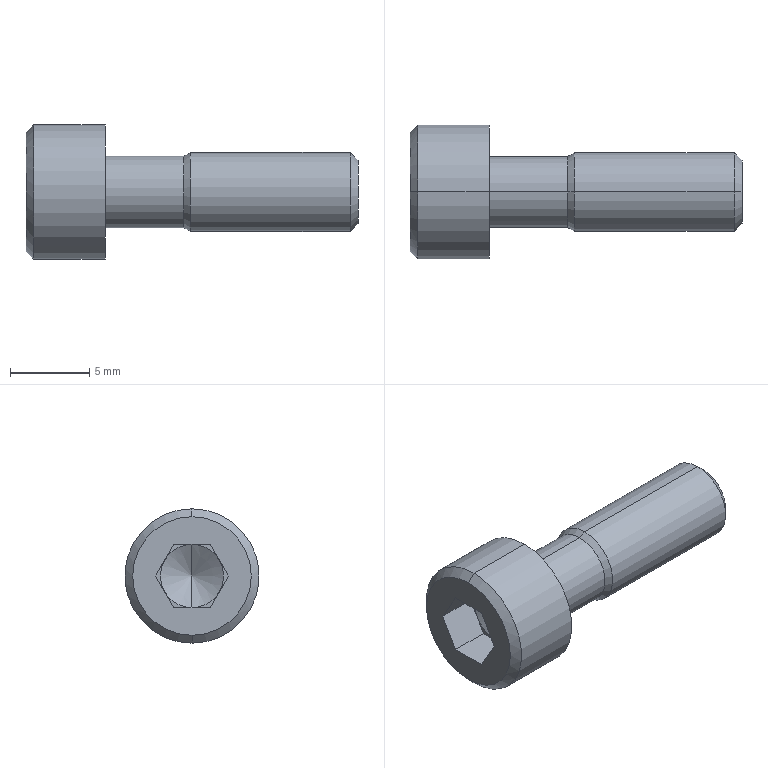Part | STEP file | 0245_Z_041_HCBST5-16_1 | 1 solid | 29 faces | box 21 x 8.5 x 8.5 mm | volume 534.382 mm3 | plane 15 | cone 8 | cylinder 6 | commonest cylinder face diameters 4.509 x2 5 x2 8.5 x2